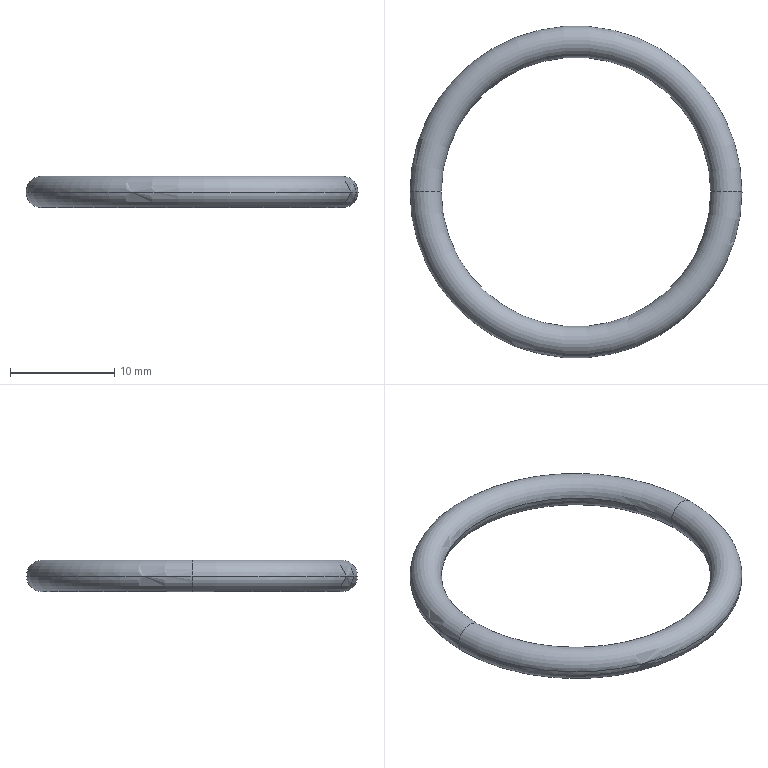Part | STEP file | ZXCOMPANY_A782D-L-09 | 1 solid | 4 faces | box 31.8 x 31.8 x 3 mm | volume 639.55 mm3 | torus 4
STEP:
#1=CARTESIAN_POINT('',(0.,0.,0.));
#2=DIRECTION('',(0.,0.,1.));
#3=DIRECTION('',(1.,0.,0.));
#4=AXIS2_PLACEMENT_3D('',#1,#2,#3);
#5=CARTESIAN_POINT('',(-12.9,0.,0.));
#6=VERTEX_POINT('',#5);
#7=CARTESIAN_POINT('',(-15.9,0.,0.));
#8=VERTEX_POINT('',#7);
#9=CARTESIAN_POINT('',(-14.4,0.,0.));
#10=DIRECTION('',(0.,1.,0.));
#11=DIRECTION('',(1.,0.,0.));
#12=AXIS2_PLACEMENT_3D('',#9,#10,#11);
#13=CIRCLE('',#12,1.5);
#14=EDGE_CURVE('',#6,#8,#13,.T.);
#15=ORIENTED_EDGE('',*,*,#14,.T.);
#16=CARTESIAN_POINT('',(15.9,0.,0.));
#17=VERTEX_POINT('',#16);
#18=CARTESIAN_POINT('',(0.,0.,0.));
#19=DIRECTION('',(0.,0.,1.));
#20=DIRECTION('',(-1.,0.,0.));
#21=AXIS2_PLACEMENT_3D('',#18,#19,#20);
#22=CIRCLE('',#21,15.9);
#23=EDGE_CURVE('',#8,#17,#22,.T.);
#24=ORIENTED_EDGE('',*,*,#23,.T.);
#25=CARTESIAN_POINT('',(12.9,0.,0.));
#26=VERTEX_POINT('',#25);
#27=CARTESIAN_POINT('',(14.4,0.,0.));
#28=DIRECTION('',(0.,-1.,0.));
#29=DIRECTION('',(-1.,0.,0.));
#30=AXIS2_PLACEMENT_3D('',#27,#28,#29);
#31=CIRCLE('',#30,1.5);
#32=EDGE_CURVE('',#26,#17,#31,.T.);
#33=ORIENTED_EDGE('',*,*,#32,.F.);
#34=CARTESIAN_POINT('',(0.,0.,0.));
#35=DIRECTION('',(0.,0.,1.));
#36=DIRECTION('',(-1.,0.,0.));
#37=AXIS2_PLACEMENT_3D('',#34,#35,#36);
#38=CIRCLE('',#37,12.9);
#39=EDGE_CURVE('',#6,#26,#38,.T.);
#40=ORIENTED_EDGE('',*,*,#39,.F.);
#41=EDGE_LOOP('',(#15,#24,#33,#40));
#42=FACE_OUTER_BOUND('',#41,.F.);
#43=CARTESIAN_POINT('',(0.,0.,0.));
#44=DIRECTION('',(0.,0.,1.));
#45=DIRECTION('',(-1.,0.,0.));
#46=AXIS2_PLACEMENT_3D('',#43,#44,#45);
#47=TOROIDAL_SURFACE('',#46,14.4,1.5);
#48=ADVANCED_FACE('',(#42),#47,.T.);
#49=ORIENTED_EDGE('',*,*,#14,.F.);
#50=CARTESIAN_POINT('',(0.,0.,0.));
#51=DIRECTION('',(0.,0.,-1.));
#52=DIRECTION('',(-1.,0.,0.));
#53=AXIS2_PLACEMENT_3D('',#50,#51,#52);
#54=CIRCLE('',#53,12.9);
#55=EDGE_CURVE('',#6,#26,#54,.T.);
#56=ORIENTED_EDGE('',*,*,#55,.T.);
#57=ORIENTED_EDGE('',*,*,#32,.T.);
#58=CARTESIAN_POINT('',(0.,0.,0.));
#59=DIRECTION('',(0.,0.,-1.));
#60=DIRECTION('',(-1.,0.,0.));
#61=AXIS2_PLACEMENT_3D('',#58,#59,#60);
#62=CIRCLE('',#61,15.9);
#63=EDGE_CURVE('',#8,#17,#62,.T.);
#64=ORIENTED_EDGE('',*,*,#63,.F.);
#65=EDGE_LOOP('',(#49,#56,#57,#64));
#66=FACE_OUTER_BOUND('',#65,.F.);
#67=CARTESIAN_POINT('',(0.,0.,0.));
#68=DIRECTION('',(0.,0.,1.));
#69=DIRECTION('',(-1.,0.,0.));
#70=AXIS2_PLACEMENT_3D('',#67,#68,#69);
#71=TOROIDAL_SURFACE('',#70,14.4,1.5);
#72=ADVANCED_FACE('',(#66),#71,.T.);
#73=CARTESIAN_POINT('',(-14.4,0.,0.));
#74=DIRECTION('',(0.,1.,0.));
#75=DIRECTION('',(-1.,0.,0.));
#76=AXIS2_PLACEMENT_3D('',#73,#74,#75);
#77=CIRCLE('',#76,1.5);
#78=EDGE_CURVE('',#8,#6,#77,.T.);
#79=ORIENTED_EDGE('',*,*,#78,.F.);
#80=ORIENTED_EDGE('',*,*,#63,.T.);
#81=CARTESIAN_POINT('',(14.4,0.,0.));
#82=DIRECTION('',(0.,-1.,0.));
#83=DIRECTION('',(1.,0.,0.));
#84=AXIS2_PLACEMENT_3D('',#81,#82,#83);
#85=CIRCLE('',#84,1.5);
#86=EDGE_CURVE('',#17,#26,#85,.T.);
#87=ORIENTED_EDGE('',*,*,#86,.T.);
#88=ORIENTED_EDGE('',*,*,#55,.F.);
#89=EDGE_LOOP('',(#79,#80,#87,#88));
#90=FACE_OUTER_BOUND('',#89,.F.);
#91=CARTESIAN_POINT('',(0.,0.,0.));
#92=DIRECTION('',(0.,0.,1.));
#93=DIRECTION('',(-1.,0.,0.));
#94=AXIS2_PLACEMENT_3D('',#91,#92,#93);
#95=TOROIDAL_SURFACE('',#94,14.4,1.5);
#96=ADVANCED_FACE('',(#90),#95,.T.);
#97=ORIENTED_EDGE('',*,*,#78,.T.);
#98=ORIENTED_EDGE('',*,*,#39,.T.);
#99=ORIENTED_EDGE('',*,*,#86,.F.);
#100=ORIENTED_EDGE('',*,*,#23,.F.);
#101=EDGE_LOOP('',(#97,#98,#99,#100));
#102=FACE_OUTER_BOUND('',#101,.F.);
#103=CARTESIAN_POINT('',(0.,0.,0.));
#104=DIRECTION('',(0.,0.,1.));
#105=DIRECTION('',(-1.,0.,0.));
#106=AXIS2_PLACEMENT_3D('',#103,#104,#105);
#107=TOROIDAL_SURFACE('',#106,14.4,1.5);
#108=ADVANCED_FACE('',(#102),#107,.T.);
#109=CLOSED_SHELL('',(#48,#72,#96,#108));
#110=MANIFOLD_SOLID_BREP('',#109);
#111=(LENGTH_UNIT()NAMED_UNIT(*)SI_UNIT(.MILLI.,.METRE.));
#112=UNCERTAINTY_MEASURE_WITH_UNIT(LENGTH_MEASURE(0.004507),#111,'','');
#113=(NAMED_UNIT(*)PLANE_ANGLE_UNIT()SI_UNIT($,.RADIAN.));
#114=PLANE_ANGLE_MEASURE_WITH_UNIT(PLANE_ANGLE_MEASURE(0.01745),#113);
#115=(CONVERSION_BASED_UNIT('DEGREE',#114)NAMED_UNIT(*)PLANE_ANGLE_UNIT());
#116=(NAMED_UNIT(*)SI_UNIT($,.STERADIAN.)SOLID_ANGLE_UNIT());
#117=(GEOMETRIC_REPRESENTATION_CONTEXT(3)GLOBAL_UNCERTAINTY_ASSIGNED_CONTEXT((#112))GLOBAL_UNIT_ASSIGNED_CONTEXT((#111,#115,#116))REPRESENTATION_CONTEXT('',''));
#118=ADVANCED_BREP_SHAPE_REPRESENTATION('',(#4,#110),#117);